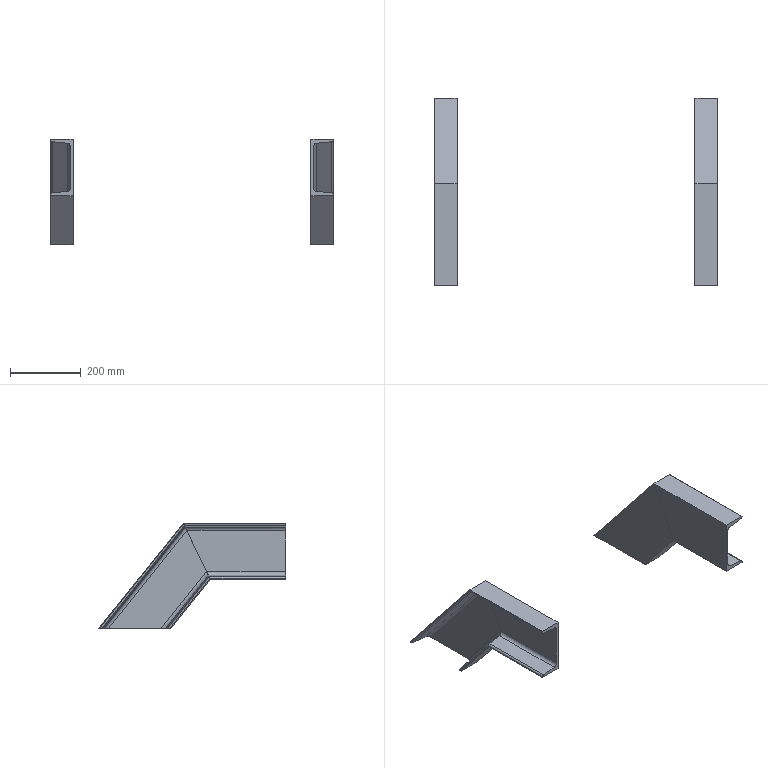Part | STEP file | E3-计量楼梯主体_Default<As Machined> | 4 solids | 56 faces | box 800 x 530 x 300 mm | volume 2341244 mm3 | plane 40 | cylinder 16 | commonest cylinder face diameters 10 x8 20 x8